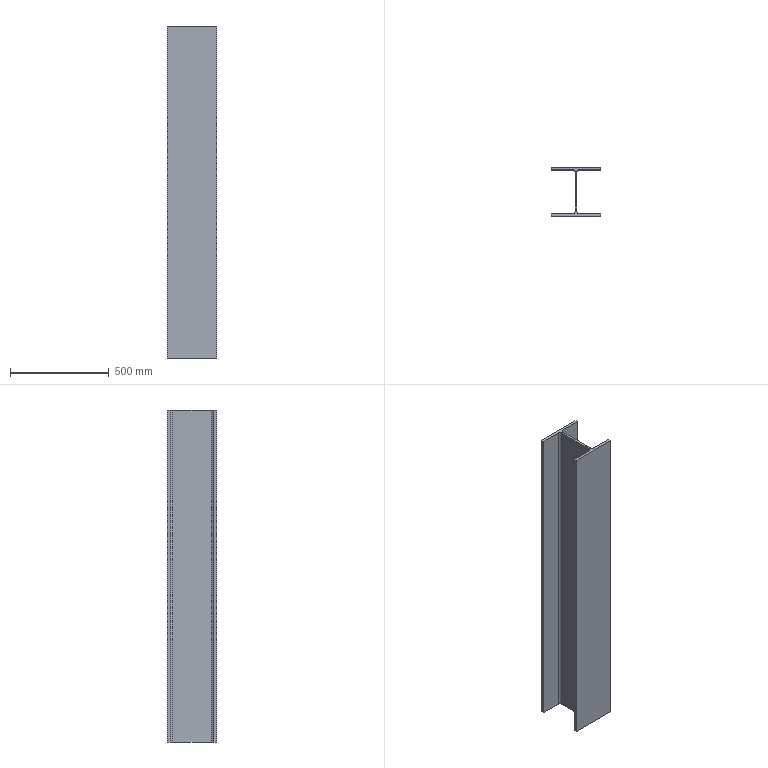Part | SolidWorks | features Extrusion 1 | 1 solid | 18 faces | box 250 x 250 x 1681 mm | volume 15369502 mm3 | plane 14 | cylinder 4 | commonest cylinder face diameters 26 x4
STEP:
#1=CARTESIAN_POINT('',(0.,14.,0.));
#2=VERTEX_POINT('',#1);
#3=CARTESIAN_POINT('',(0.,0.,0.));
#4=VERTEX_POINT('',#3);
#5=CARTESIAN_POINT('',(0.,14.,0.));
#6=DIRECTION('',(0.,-1.,0.));
#7=VECTOR('',#6,1000.);
#8=LINE('',#5,#7);
#9=EDGE_CURVE('',#2,#4,#8,.T.);
#10=ORIENTED_EDGE('',*,*,#9,.T.);
#11=CARTESIAN_POINT('',(0.,0.,1681.));
#12=VERTEX_POINT('',#11);
#13=CARTESIAN_POINT('',(0.,0.,1681.));
#14=DIRECTION('',(0.,0.,-1.));
#15=VECTOR('',#14,1000.);
#16=LINE('',#13,#15);
#17=EDGE_CURVE('',#12,#4,#16,.T.);
#18=ORIENTED_EDGE('',*,*,#17,.F.);
#19=CARTESIAN_POINT('',(0.,14.,1681.));
#20=VERTEX_POINT('',#19);
#21=CARTESIAN_POINT('',(0.,14.,1681.));
#22=DIRECTION('',(0.,-1.,0.));
#23=VECTOR('',#22,1000.);
#24=LINE('',#21,#23);
#25=EDGE_CURVE('',#20,#12,#24,.T.);
#26=ORIENTED_EDGE('',*,*,#25,.F.);
#27=CARTESIAN_POINT('',(0.,14.,1681.));
#28=DIRECTION('',(0.,0.,-1.));
#29=VECTOR('',#28,1000.);
#30=LINE('',#27,#29);
#31=EDGE_CURVE('',#20,#2,#30,.T.);
#32=ORIENTED_EDGE('',*,*,#31,.T.);
#33=EDGE_LOOP('',(#10,#18,#26,#32));
#34=FACE_OUTER_BOUND('',#33,.T.);
#35=CARTESIAN_POINT('',(0.,14.,1681.));
#36=DIRECTION('',(1.,0.,0.));
#37=DIRECTION('',(0.,1.,0.));
#38=AXIS2_PLACEMENT_3D('',#35,#36,#37);
#39=PLANE('',#38);
#40=ADVANCED_FACE('',(#34),#39,.F.);
#41=CARTESIAN_POINT('',(250.,0.,0.));
#42=VERTEX_POINT('',#41);
#43=CARTESIAN_POINT('',(0.,0.,0.));
#44=DIRECTION('',(1.,0.,0.));
#45=VECTOR('',#44,1000.);
#46=LINE('',#43,#45);
#47=EDGE_CURVE('',#4,#42,#46,.T.);
#48=ORIENTED_EDGE('',*,*,#47,.T.);
#49=CARTESIAN_POINT('',(250.,0.,1681.));
#50=VERTEX_POINT('',#49);
#51=CARTESIAN_POINT('',(250.,0.,1681.));
#52=DIRECTION('',(0.,0.,-1.));
#53=VECTOR('',#52,1000.);
#54=LINE('',#51,#53);
#55=EDGE_CURVE('',#50,#42,#54,.T.);
#56=ORIENTED_EDGE('',*,*,#55,.F.);
#57=CARTESIAN_POINT('',(0.,0.,1681.));
#58=DIRECTION('',(1.,0.,0.));
#59=VECTOR('',#58,1000.);
#60=LINE('',#57,#59);
#61=EDGE_CURVE('',#12,#50,#60,.T.);
#62=ORIENTED_EDGE('',*,*,#61,.F.);
#63=ORIENTED_EDGE('',*,*,#17,.T.);
#64=EDGE_LOOP('',(#48,#56,#62,#63));
#65=FACE_OUTER_BOUND('',#64,.T.);
#66=CARTESIAN_POINT('',(0.,0.,1681.));
#67=DIRECTION('',(0.,1.,0.));
#68=DIRECTION('',(-1.,0.,0.));
#69=AXIS2_PLACEMENT_3D('',#66,#67,#68);
#70=PLANE('',#69);
#71=ADVANCED_FACE('',(#65),#70,.F.);
#72=CARTESIAN_POINT('',(250.,14.,0.));
#73=VERTEX_POINT('',#72);
#74=CARTESIAN_POINT('',(250.,0.,0.));
#75=DIRECTION('',(0.,1.,0.));
#76=VECTOR('',#75,1000.);
#77=LINE('',#74,#76);
#78=EDGE_CURVE('',#42,#73,#77,.T.);
#79=ORIENTED_EDGE('',*,*,#78,.T.);
#80=CARTESIAN_POINT('',(250.,14.,1681.));
#81=VERTEX_POINT('',#80);
#82=CARTESIAN_POINT('',(250.,14.,1681.));
#83=DIRECTION('',(0.,0.,-1.));
#84=VECTOR('',#83,1000.);
#85=LINE('',#82,#84);
#86=EDGE_CURVE('',#81,#73,#85,.T.);
#87=ORIENTED_EDGE('',*,*,#86,.F.);
#88=CARTESIAN_POINT('',(250.,0.,1681.));
#89=DIRECTION('',(0.,1.,0.));
#90=VECTOR('',#89,1000.);
#91=LINE('',#88,#90);
#92=EDGE_CURVE('',#50,#81,#91,.T.);
#93=ORIENTED_EDGE('',*,*,#92,.F.);
#94=ORIENTED_EDGE('',*,*,#55,.T.);
#95=EDGE_LOOP('',(#79,#87,#93,#94));
#96=FACE_OUTER_BOUND('',#95,.T.);
#97=CARTESIAN_POINT('',(250.,0.,1681.));
#98=DIRECTION('',(-1.,0.,0.));
#99=DIRECTION('',(0.,0.,1.));
#100=AXIS2_PLACEMENT_3D('',#97,#98,#99);
#101=PLANE('',#100);
#102=ADVANCED_FACE('',(#96),#101,.F.);
#103=CARTESIAN_POINT('',(142.5,14.,0.));
#104=VERTEX_POINT('',#103);
#105=CARTESIAN_POINT('',(250.,14.,0.));
#106=DIRECTION('',(-1.,0.,0.));
#107=VECTOR('',#106,1000.);
#108=LINE('',#105,#107);
#109=EDGE_CURVE('',#73,#104,#108,.T.);
#110=ORIENTED_EDGE('',*,*,#109,.T.);
#111=CARTESIAN_POINT('',(142.5,14.,1681.));
#112=VERTEX_POINT('',#111);
#113=CARTESIAN_POINT('',(142.5,14.,1681.));
#114=DIRECTION('',(0.,0.,-1.));
#115=VECTOR('',#114,1000.);
#116=LINE('',#113,#115);
#117=EDGE_CURVE('',#112,#104,#116,.T.);
#118=ORIENTED_EDGE('',*,*,#117,.F.);
#119=CARTESIAN_POINT('',(250.,14.,1681.));
#120=DIRECTION('',(-1.,0.,0.));
#121=VECTOR('',#120,1000.);
#122=LINE('',#119,#121);
#123=EDGE_CURVE('',#81,#112,#122,.T.);
#124=ORIENTED_EDGE('',*,*,#123,.F.);
#125=ORIENTED_EDGE('',*,*,#86,.T.);
#126=EDGE_LOOP('',(#110,#118,#124,#125));
#127=FACE_OUTER_BOUND('',#126,.T.);
#128=CARTESIAN_POINT('',(250.,14.,1681.));
#129=DIRECTION('',(0.,-1.,0.));
#130=DIRECTION('',(1.,0.,0.));
#131=AXIS2_PLACEMENT_3D('',#128,#129,#130);
#132=PLANE('',#131);
#133=ADVANCED_FACE('',(#127),#132,.F.);
#134=CARTESIAN_POINT('',(129.5,27.,0.));
#135=VERTEX_POINT('',#134);
#136=CARTESIAN_POINT('',(142.5,27.,0.));
#137=DIRECTION('',(0.,0.,-1.));
#138=DIRECTION('',(-1.,0.,0.));
#139=AXIS2_PLACEMENT_3D('',#136,#137,#138);
#140=CIRCLE('',#139,13.);
#141=EDGE_CURVE('',#104,#135,#140,.T.);
#142=ORIENTED_EDGE('',*,*,#141,.T.);
#143=CARTESIAN_POINT('',(129.5,27.,1681.));
#144=VERTEX_POINT('',#143);
#145=CARTESIAN_POINT('',(129.5,27.,1681.));
#146=DIRECTION('',(0.,0.,-1.));
#147=VECTOR('',#146,1000.);
#148=LINE('',#145,#147);
#149=EDGE_CURVE('',#144,#135,#148,.T.);
#150=ORIENTED_EDGE('',*,*,#149,.F.);
#151=CARTESIAN_POINT('',(142.5,27.,1681.));
#152=DIRECTION('',(0.,0.,-1.));
#153=DIRECTION('',(-1.,0.,0.));
#154=AXIS2_PLACEMENT_3D('',#151,#152,#153);
#155=CIRCLE('',#154,13.);
#156=EDGE_CURVE('',#112,#144,#155,.T.);
#157=ORIENTED_EDGE('',*,*,#156,.F.);
#158=ORIENTED_EDGE('',*,*,#117,.T.);
#159=EDGE_LOOP('',(#142,#150,#157,#158));
#160=FACE_OUTER_BOUND('',#159,.T.);
#161=CARTESIAN_POINT('',(142.5,27.,1681.));
#162=DIRECTION('',(0.,0.,-1.));
#163=DIRECTION('',(-1.,0.,0.));
#164=AXIS2_PLACEMENT_3D('',#161,#162,#163);
#165=CYLINDRICAL_SURFACE('',#164,13.);
#166=ADVANCED_FACE('',(#160),#165,.F.);
#167=CARTESIAN_POINT('',(129.5,223.,0.));
#168=VERTEX_POINT('',#167);
#169=CARTESIAN_POINT('',(129.5,27.,0.));
#170=DIRECTION('',(0.,1.,0.));
#171=VECTOR('',#170,1000.);
#172=LINE('',#169,#171);
#173=EDGE_CURVE('',#135,#168,#172,.T.);
#174=ORIENTED_EDGE('',*,*,#173,.T.);
#175=CARTESIAN_POINT('',(129.5,223.,1681.));
#176=VERTEX_POINT('',#175);
#177=CARTESIAN_POINT('',(129.5,223.,1681.));
#178=DIRECTION('',(0.,0.,-1.));
#179=VECTOR('',#178,1000.);
#180=LINE('',#177,#179);
#181=EDGE_CURVE('',#176,#168,#180,.T.);
#182=ORIENTED_EDGE('',*,*,#181,.F.);
#183=CARTESIAN_POINT('',(129.5,27.,1681.));
#184=DIRECTION('',(0.,1.,0.));
#185=VECTOR('',#184,1000.);
#186=LINE('',#183,#185);
#187=EDGE_CURVE('',#144,#176,#186,.T.);
#188=ORIENTED_EDGE('',*,*,#187,.F.);
#189=ORIENTED_EDGE('',*,*,#149,.T.);
#190=EDGE_LOOP('',(#174,#182,#188,#189));
#191=FACE_OUTER_BOUND('',#190,.T.);
#192=CARTESIAN_POINT('',(129.5,27.,1681.));
#193=DIRECTION('',(-1.,0.,0.));
#194=DIRECTION('',(0.,-1.,0.));
#195=AXIS2_PLACEMENT_3D('',#192,#193,#194);
#196=PLANE('',#195);
#197=ADVANCED_FACE('',(#191),#196,.F.);
#198=CARTESIAN_POINT('',(142.5,236.,0.));
#199=VERTEX_POINT('',#198);
#200=CARTESIAN_POINT('',(142.5,223.,0.));
#201=DIRECTION('',(0.,0.,-1.));
#202=DIRECTION('',(-1.,0.,0.));
#203=AXIS2_PLACEMENT_3D('',#200,#201,#202);
#204=CIRCLE('',#203,13.);
#205=EDGE_CURVE('',#168,#199,#204,.T.);
#206=ORIENTED_EDGE('',*,*,#205,.T.);
#207=CARTESIAN_POINT('',(142.5,236.,1681.));
#208=VERTEX_POINT('',#207);
#209=CARTESIAN_POINT('',(142.5,236.,1681.));
#210=DIRECTION('',(0.,0.,-1.));
#211=VECTOR('',#210,1000.);
#212=LINE('',#209,#211);
#213=EDGE_CURVE('',#208,#199,#212,.T.);
#214=ORIENTED_EDGE('',*,*,#213,.F.);
#215=CARTESIAN_POINT('',(142.5,223.,1681.));
#216=DIRECTION('',(0.,0.,-1.));
#217=DIRECTION('',(-1.,0.,0.));
#218=AXIS2_PLACEMENT_3D('',#215,#216,#217);
#219=CIRCLE('',#218,13.);
#220=EDGE_CURVE('',#176,#208,#219,.T.);
#221=ORIENTED_EDGE('',*,*,#220,.F.);
#222=ORIENTED_EDGE('',*,*,#181,.T.);
#223=EDGE_LOOP('',(#206,#214,#221,#222));
#224=FACE_OUTER_BOUND('',#223,.T.);
#225=CARTESIAN_POINT('',(142.5,223.,1681.));
#226=DIRECTION('',(0.,0.,-1.));
#227=DIRECTION('',(-1.,0.,0.));
#228=AXIS2_PLACEMENT_3D('',#225,#226,#227);
#229=CYLINDRICAL_SURFACE('',#228,13.);
#230=ADVANCED_FACE('',(#224),#229,.F.);
#231=CARTESIAN_POINT('',(250.,236.,0.));
#232=VERTEX_POINT('',#231);
#233=CARTESIAN_POINT('',(142.5,236.,0.));
#234=DIRECTION('',(1.,0.,0.));
#235=VECTOR('',#234,1000.);
#236=LINE('',#233,#235);
#237=EDGE_CURVE('',#199,#232,#236,.T.);
#238=ORIENTED_EDGE('',*,*,#237,.T.);
#239=CARTESIAN_POINT('',(250.,236.,1681.));
#240=VERTEX_POINT('',#239);
#241=CARTESIAN_POINT('',(250.,236.,1681.));
#242=DIRECTION('',(0.,0.,-1.));
#243=VECTOR('',#242,1000.);
#244=LINE('',#241,#243);
#245=EDGE_CURVE('',#240,#232,#244,.T.);
#246=ORIENTED_EDGE('',*,*,#245,.F.);
#247=CARTESIAN_POINT('',(142.5,236.,1681.));
#248=DIRECTION('',(1.,0.,0.));
#249=VECTOR('',#248,1000.);
#250=LINE('',#247,#249);
#251=EDGE_CURVE('',#208,#240,#250,.T.);
#252=ORIENTED_EDGE('',*,*,#251,.F.);
#253=ORIENTED_EDGE('',*,*,#213,.T.);
#254=EDGE_LOOP('',(#238,#246,#252,#253));
#255=FACE_OUTER_BOUND('',#254,.T.);
#256=CARTESIAN_POINT('',(142.5,236.,1681.));
#257=DIRECTION('',(0.,1.,0.));
#258=DIRECTION('',(0.,0.,1.));
#259=AXIS2_PLACEMENT_3D('',#256,#257,#258);
#260=PLANE('',#259);
#261=ADVANCED_FACE('',(#255),#260,.F.);
#262=CARTESIAN_POINT('',(250.,250.,0.));
#263=VERTEX_POINT('',#262);
#264=CARTESIAN_POINT('',(250.,236.,0.));
#265=DIRECTION('',(0.,1.,0.));
#266=VECTOR('',#265,1000.);
#267=LINE('',#264,#266);
#268=EDGE_CURVE('',#232,#263,#267,.T.);
#269=ORIENTED_EDGE('',*,*,#268,.T.);
#270=CARTESIAN_POINT('',(250.,250.,1681.));
#271=VERTEX_POINT('',#270);
#272=CARTESIAN_POINT('',(250.,250.,1681.));
#273=DIRECTION('',(0.,0.,-1.));
#274=VECTOR('',#273,1000.);
#275=LINE('',#272,#274);
#276=EDGE_CURVE('',#271,#263,#275,.T.);
#277=ORIENTED_EDGE('',*,*,#276,.F.);
#278=CARTESIAN_POINT('',(250.,236.,1681.));
#279=DIRECTION('',(0.,1.,0.));
#280=VECTOR('',#279,1000.);
#281=LINE('',#278,#280);
#282=EDGE_CURVE('',#240,#271,#281,.T.);
#283=ORIENTED_EDGE('',*,*,#282,.F.);
#284=ORIENTED_EDGE('',*,*,#245,.T.);
#285=EDGE_LOOP('',(#269,#277,#283,#284));
#286=FACE_OUTER_BOUND('',#285,.T.);
#287=CARTESIAN_POINT('',(250.,236.,1681.));
#288=DIRECTION('',(-1.,0.,0.));
#289=DIRECTION('',(0.,0.,1.));
#290=AXIS2_PLACEMENT_3D('',#287,#288,#289);
#291=PLANE('',#290);
#292=ADVANCED_FACE('',(#286),#291,.F.);
#293=CARTESIAN_POINT('',(0.,250.,0.));
#294=VERTEX_POINT('',#293);
#295=CARTESIAN_POINT('',(250.,250.,0.));
#296=DIRECTION('',(-1.,0.,0.));
#297=VECTOR('',#296,1000.);
#298=LINE('',#295,#297);
#299=EDGE_CURVE('',#263,#294,#298,.T.);
#300=ORIENTED_EDGE('',*,*,#299,.T.);
#301=CARTESIAN_POINT('',(0.,250.,1681.));
#302=VERTEX_POINT('',#301);
#303=CARTESIAN_POINT('',(0.,250.,1681.));
#304=DIRECTION('',(0.,0.,-1.));
#305=VECTOR('',#304,1000.);
#306=LINE('',#303,#305);
#307=EDGE_CURVE('',#302,#294,#306,.T.);
#308=ORIENTED_EDGE('',*,*,#307,.F.);
#309=CARTESIAN_POINT('',(250.,250.,1681.));
#310=DIRECTION('',(-1.,0.,0.));
#311=VECTOR('',#310,1000.);
#312=LINE('',#309,#311);
#313=EDGE_CURVE('',#271,#302,#312,.T.);
#314=ORIENTED_EDGE('',*,*,#313,.F.);
#315=ORIENTED_EDGE('',*,*,#276,.T.);
#316=EDGE_LOOP('',(#300,#308,#314,#315));
#317=FACE_OUTER_BOUND('',#316,.T.);
#318=CARTESIAN_POINT('',(250.,250.,1681.));
#319=DIRECTION('',(0.,-1.,0.));
#320=DIRECTION('',(0.,0.,-1.));
#321=AXIS2_PLACEMENT_3D('',#318,#319,#320);
#322=PLANE('',#321);
#323=ADVANCED_FACE('',(#317),#322,.F.);
#324=CARTESIAN_POINT('',(0.,236.,0.));
#325=VERTEX_POINT('',#324);
#326=CARTESIAN_POINT('',(0.,250.,0.));
#327=DIRECTION('',(0.,-1.,0.));
#328=VECTOR('',#327,1000.);
#329=LINE('',#326,#328);
#330=EDGE_CURVE('',#294,#325,#329,.T.);
#331=ORIENTED_EDGE('',*,*,#330,.T.);
#332=CARTESIAN_POINT('',(0.,236.,1681.));
#333=VERTEX_POINT('',#332);
#334=CARTESIAN_POINT('',(0.,236.,1681.));
#335=DIRECTION('',(0.,0.,-1.));
#336=VECTOR('',#335,1000.);
#337=LINE('',#334,#336);
#338=EDGE_CURVE('',#333,#325,#337,.T.);
#339=ORIENTED_EDGE('',*,*,#338,.F.);
#340=CARTESIAN_POINT('',(0.,250.,1681.));
#341=DIRECTION('',(0.,-1.,0.));
#342=VECTOR('',#341,1000.);
#343=LINE('',#340,#342);
#344=EDGE_CURVE('',#302,#333,#343,.T.);
#345=ORIENTED_EDGE('',*,*,#344,.F.);
#346=ORIENTED_EDGE('',*,*,#307,.T.);
#347=EDGE_LOOP('',(#331,#339,#345,#346));
#348=FACE_OUTER_BOUND('',#347,.T.);
#349=CARTESIAN_POINT('',(0.,250.,1681.));
#350=DIRECTION('',(1.,0.,0.));
#351=DIRECTION('',(0.,1.,0.));
#352=AXIS2_PLACEMENT_3D('',#349,#350,#351);
#353=PLANE('',#352);
#354=ADVANCED_FACE('',(#348),#353,.F.);
#355=CARTESIAN_POINT('',(107.5,236.,0.));
#356=VERTEX_POINT('',#355);
#357=CARTESIAN_POINT('',(0.,236.,0.));
#358=DIRECTION('',(1.,0.,0.));
#359=VECTOR('',#358,1000.);
#360=LINE('',#357,#359);
#361=EDGE_CURVE('',#325,#356,#360,.T.);
#362=ORIENTED_EDGE('',*,*,#361,.T.);
#363=CARTESIAN_POINT('',(107.5,236.,1681.));
#364=VERTEX_POINT('',#363);
#365=CARTESIAN_POINT('',(107.5,236.,1681.));
#366=DIRECTION('',(0.,0.,-1.));
#367=VECTOR('',#366,1000.);
#368=LINE('',#365,#367);
#369=EDGE_CURVE('',#364,#356,#368,.T.);
#370=ORIENTED_EDGE('',*,*,#369,.F.);
#371=CARTESIAN_POINT('',(0.,236.,1681.));
#372=DIRECTION('',(1.,0.,0.));
#373=VECTOR('',#372,1000.);
#374=LINE('',#371,#373);
#375=EDGE_CURVE('',#333,#364,#374,.T.);
#376=ORIENTED_EDGE('',*,*,#375,.F.);
#377=ORIENTED_EDGE('',*,*,#338,.T.);
#378=EDGE_LOOP('',(#362,#370,#376,#377));
#379=FACE_OUTER_BOUND('',#378,.T.);
#380=CARTESIAN_POINT('',(0.,236.,1681.));
#381=DIRECTION('',(0.,1.,0.));
#382=DIRECTION('',(-1.,0.,0.));
#383=AXIS2_PLACEMENT_3D('',#380,#381,#382);
#384=PLANE('',#383);
#385=ADVANCED_FACE('',(#379),#384,.F.);
#386=CARTESIAN_POINT('',(120.5,223.,0.));
#387=VERTEX_POINT('',#386);
#388=CARTESIAN_POINT('',(107.5,223.,0.));
#389=DIRECTION('',(0.,0.,-1.));
#390=DIRECTION('',(-1.,0.,0.));
#391=AXIS2_PLACEMENT_3D('',#388,#389,#390);
#392=CIRCLE('',#391,13.);
#393=EDGE_CURVE('',#356,#387,#392,.T.);
#394=ORIENTED_EDGE('',*,*,#393,.T.);
#395=CARTESIAN_POINT('',(120.5,223.,1681.));
#396=VERTEX_POINT('',#395);
#397=CARTESIAN_POINT('',(120.5,223.,1681.));
#398=DIRECTION('',(0.,0.,-1.));
#399=VECTOR('',#398,1000.);
#400=LINE('',#397,#399);
#401=EDGE_CURVE('',#396,#387,#400,.T.);
#402=ORIENTED_EDGE('',*,*,#401,.F.);
#403=CARTESIAN_POINT('',(107.5,223.,1681.));
#404=DIRECTION('',(0.,0.,-1.));
#405=DIRECTION('',(-1.,0.,0.));
#406=AXIS2_PLACEMENT_3D('',#403,#404,#405);
#407=CIRCLE('',#406,13.);
#408=EDGE_CURVE('',#364,#396,#407,.T.);
#409=ORIENTED_EDGE('',*,*,#408,.F.);
#410=ORIENTED_EDGE('',*,*,#369,.T.);
#411=EDGE_LOOP('',(#394,#402,#409,#410));
#412=FACE_OUTER_BOUND('',#411,.T.);
#413=CARTESIAN_POINT('',(107.5,223.,1681.));
#414=DIRECTION('',(0.,0.,-1.));
#415=DIRECTION('',(-1.,0.,0.));
#416=AXIS2_PLACEMENT_3D('',#413,#414,#415);
#417=CYLINDRICAL_SURFACE('',#416,13.);
#418=ADVANCED_FACE('',(#412),#417,.F.);
#419=CARTESIAN_POINT('',(120.5,27.,0.));
#420=VERTEX_POINT('',#419);
#421=CARTESIAN_POINT('',(120.5,223.,0.));
#422=DIRECTION('',(0.,-1.,0.));
#423=VECTOR('',#422,1000.);
#424=LINE('',#421,#423);
#425=EDGE_CURVE('',#387,#420,#424,.T.);
#426=ORIENTED_EDGE('',*,*,#425,.T.);
#427=CARTESIAN_POINT('',(120.5,27.,1681.));
#428=VERTEX_POINT('',#427);
#429=CARTESIAN_POINT('',(120.5,27.,1681.));
#430=DIRECTION('',(0.,0.,-1.));
#431=VECTOR('',#430,1000.);
#432=LINE('',#429,#431);
#433=EDGE_CURVE('',#428,#420,#432,.T.);
#434=ORIENTED_EDGE('',*,*,#433,.F.);
#435=CARTESIAN_POINT('',(120.5,223.,1681.));
#436=DIRECTION('',(0.,-1.,0.));
#437=VECTOR('',#436,1000.);
#438=LINE('',#435,#437);
#439=EDGE_CURVE('',#396,#428,#438,.T.);
#440=ORIENTED_EDGE('',*,*,#439,.F.);
#441=ORIENTED_EDGE('',*,*,#401,.T.);
#442=EDGE_LOOP('',(#426,#434,#440,#441));
#443=FACE_OUTER_BOUND('',#442,.T.);
#444=CARTESIAN_POINT('',(120.5,223.,1681.));
#445=DIRECTION('',(1.,0.,0.));
#446=DIRECTION('',(0.,1.,0.));
#447=AXIS2_PLACEMENT_3D('',#444,#445,#446);
#448=PLANE('',#447);
#449=ADVANCED_FACE('',(#443),#448,.F.);
#450=CARTESIAN_POINT('',(107.5,14.,0.));
#451=VERTEX_POINT('',#450);
#452=CARTESIAN_POINT('',(107.5,27.,0.));
#453=DIRECTION('',(0.,0.,-1.));
#454=DIRECTION('',(-1.,0.,0.));
#455=AXIS2_PLACEMENT_3D('',#452,#453,#454);
#456=CIRCLE('',#455,13.);
#457=EDGE_CURVE('',#420,#451,#456,.T.);
#458=ORIENTED_EDGE('',*,*,#457,.T.);
#459=CARTESIAN_POINT('',(107.5,14.,1681.));
#460=VERTEX_POINT('',#459);
#461=CARTESIAN_POINT('',(107.5,14.,1681.));
#462=DIRECTION('',(0.,0.,-1.));
#463=VECTOR('',#462,1000.);
#464=LINE('',#461,#463);
#465=EDGE_CURVE('',#460,#451,#464,.T.);
#466=ORIENTED_EDGE('',*,*,#465,.F.);
#467=CARTESIAN_POINT('',(107.5,27.,1681.));
#468=DIRECTION('',(0.,0.,-1.));
#469=DIRECTION('',(-1.,0.,0.));
#470=AXIS2_PLACEMENT_3D('',#467,#468,#469);
#471=CIRCLE('',#470,13.);
#472=EDGE_CURVE('',#428,#460,#471,.T.);
#473=ORIENTED_EDGE('',*,*,#472,.F.);
#474=ORIENTED_EDGE('',*,*,#433,.T.);
#475=EDGE_LOOP('',(#458,#466,#473,#474));
#476=FACE_OUTER_BOUND('',#475,.T.);
#477=CARTESIAN_POINT('',(107.5,27.,1681.));
#478=DIRECTION('',(0.,0.,-1.));
#479=DIRECTION('',(-1.,0.,0.));
#480=AXIS2_PLACEMENT_3D('',#477,#478,#479);
#481=CYLINDRICAL_SURFACE('',#480,13.);
#482=ADVANCED_FACE('',(#476),#481,.F.);
#483=CARTESIAN_POINT('',(107.5,14.,0.));
#484=DIRECTION('',(-1.,0.,0.));
#485=VECTOR('',#484,1000.);
#486=LINE('',#483,#485);
#487=EDGE_CURVE('',#451,#2,#486,.T.);
#488=ORIENTED_EDGE('',*,*,#487,.T.);
#489=ORIENTED_EDGE('',*,*,#31,.F.);
#490=CARTESIAN_POINT('',(107.5,14.,1681.));
#491=DIRECTION('',(-1.,0.,0.));
#492=VECTOR('',#491,1000.);
#493=LINE('',#490,#492);
#494=EDGE_CURVE('',#460,#20,#493,.T.);
#495=ORIENTED_EDGE('',*,*,#494,.F.);
#496=ORIENTED_EDGE('',*,*,#465,.T.);
#497=EDGE_LOOP('',(#488,#489,#495,#496));
#498=FACE_OUTER_BOUND('',#497,.T.);
#499=CARTESIAN_POINT('',(107.5,14.,1681.));
#500=DIRECTION('',(0.,-1.,0.));
#501=DIRECTION('',(1.,0.,0.));
#502=AXIS2_PLACEMENT_3D('',#499,#500,#501);
#503=PLANE('',#502);
#504=ADVANCED_FACE('',(#498),#503,.F.);
#505=ORIENTED_EDGE('',*,*,#25,.T.);
#506=ORIENTED_EDGE('',*,*,#61,.T.);
#507=ORIENTED_EDGE('',*,*,#92,.T.);
#508=ORIENTED_EDGE('',*,*,#123,.T.);
#509=ORIENTED_EDGE('',*,*,#156,.T.);
#510=ORIENTED_EDGE('',*,*,#187,.T.);
#511=ORIENTED_EDGE('',*,*,#220,.T.);
#512=ORIENTED_EDGE('',*,*,#251,.T.);
#513=ORIENTED_EDGE('',*,*,#282,.T.);
#514=ORIENTED_EDGE('',*,*,#313,.T.);
#515=ORIENTED_EDGE('',*,*,#344,.T.);
#516=ORIENTED_EDGE('',*,*,#375,.T.);
#517=ORIENTED_EDGE('',*,*,#408,.T.);
#518=ORIENTED_EDGE('',*,*,#439,.T.);
#519=ORIENTED_EDGE('',*,*,#472,.T.);
#520=ORIENTED_EDGE('',*,*,#494,.T.);
#521=EDGE_LOOP('',(#505,#506,#507,#508,#509,#510,#511,#512,#513,#514,#515,#516,#517,#518,#519,#520));
#522=FACE_OUTER_BOUND('',#521,.T.);
#523=CARTESIAN_POINT('',(142.5,27.,1681.));
#524=DIRECTION('',(0.,0.,-1.));
#525=DIRECTION('',(-1.,0.,0.));
#526=AXIS2_PLACEMENT_3D('',#523,#524,#525);
#527=PLANE('',#526);
#528=ADVANCED_FACE('',(#522),#527,.F.);
#529=ORIENTED_EDGE('',*,*,#9,.F.);
#530=ORIENTED_EDGE('',*,*,#487,.F.);
#531=ORIENTED_EDGE('',*,*,#457,.F.);
#532=ORIENTED_EDGE('',*,*,#425,.F.);
#533=ORIENTED_EDGE('',*,*,#393,.F.);
#534=ORIENTED_EDGE('',*,*,#361,.F.);
#535=ORIENTED_EDGE('',*,*,#330,.F.);
#536=ORIENTED_EDGE('',*,*,#299,.F.);
#537=ORIENTED_EDGE('',*,*,#268,.F.);
#538=ORIENTED_EDGE('',*,*,#237,.F.);
#539=ORIENTED_EDGE('',*,*,#205,.F.);
#540=ORIENTED_EDGE('',*,*,#173,.F.);
#541=ORIENTED_EDGE('',*,*,#141,.F.);
#542=ORIENTED_EDGE('',*,*,#109,.F.);
#543=ORIENTED_EDGE('',*,*,#78,.F.);
#544=ORIENTED_EDGE('',*,*,#47,.F.);
#545=EDGE_LOOP('',(#529,#530,#531,#532,#533,#534,#535,#536,#537,#538,#539,#540,#541,#542,#543,#544));
#546=FACE_OUTER_BOUND('',#545,.T.);
#547=CARTESIAN_POINT('',(142.5,27.,0.));
#548=DIRECTION('',(0.,0.,-1.));
#549=DIRECTION('',(-1.,0.,0.));
#550=AXIS2_PLACEMENT_3D('',#547,#548,#549);
#551=PLANE('',#550);
#552=ADVANCED_FACE('',(#546),#551,.T.);
#553=CLOSED_SHELL('',(#40,#71,#102,#133,#166,#197,#230,#261,#292,#323,#354,#385,#418,#449,#482,#504,#528,#552));
#554=MANIFOLD_SOLID_BREP('',#553);
#555=CARTESIAN_POINT('',(0.,0.,0.));
#556=DIRECTION('',(0.,0.,1.));
#557=DIRECTION('',(1.,0.,0.));
#558=AXIS2_PLACEMENT_3D('',#555,#556,#557);
#559=(LENGTH_UNIT()NAMED_UNIT(*)SI_UNIT(.MILLI.,.METRE.));
#560=UNCERTAINTY_MEASURE_WITH_UNIT(LENGTH_MEASURE(0.00001),#559,'','');
#561=(NAMED_UNIT(*)PLANE_ANGLE_UNIT()SI_UNIT($,.RADIAN.));
#562=(NAMED_UNIT(*)SI_UNIT($,.STERADIAN.)SOLID_ANGLE_UNIT());
#563=(GEOMETRIC_REPRESENTATION_CONTEXT(3)GLOBAL_UNCERTAINTY_ASSIGNED_CONTEXT((#560))GLOBAL_UNIT_ASSIGNED_CONTEXT((#559,#561,#562))REPRESENTATION_CONTEXT('',''));
#564=ADVANCED_BREP_SHAPE_REPRESENTATION('',(#554,#558),#563);